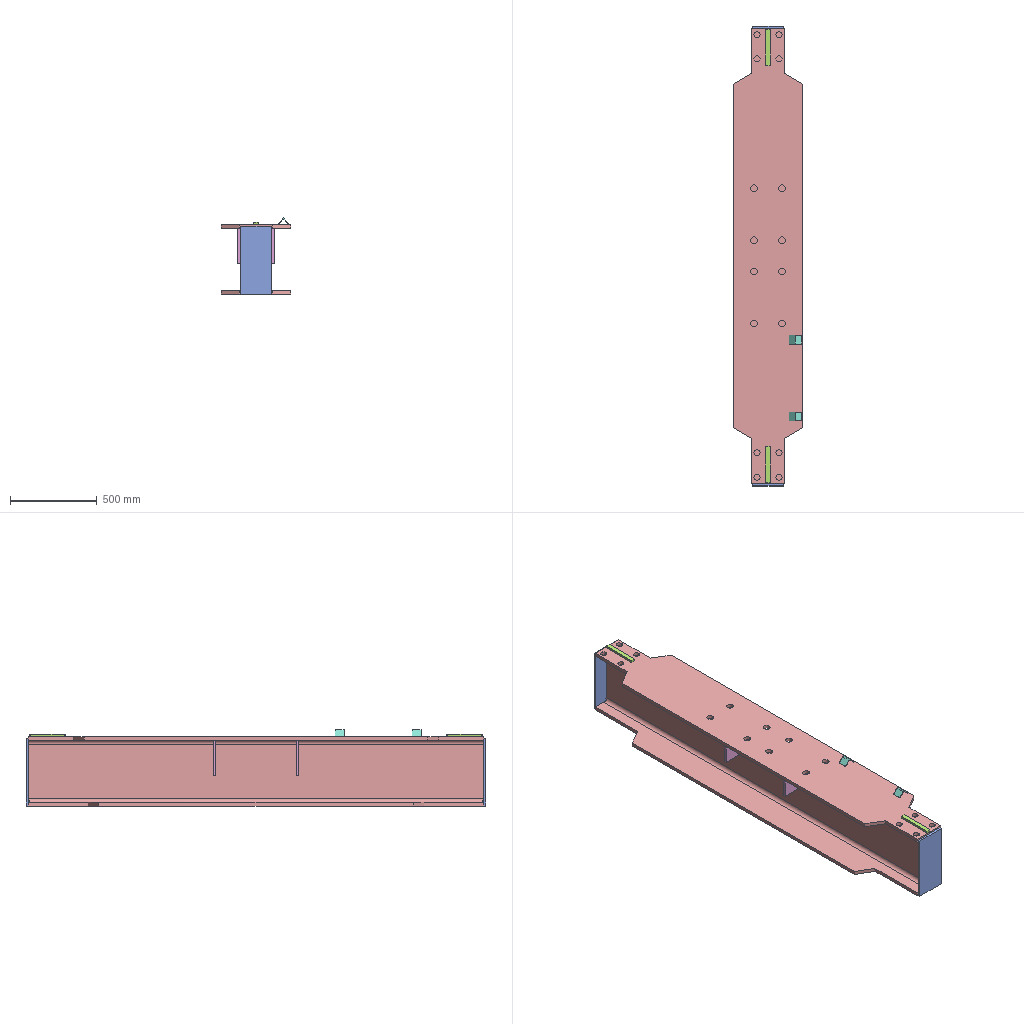Assembly | SolidWorks | 5 different items | 11 placed | box 400 x 2649 x 438 mm
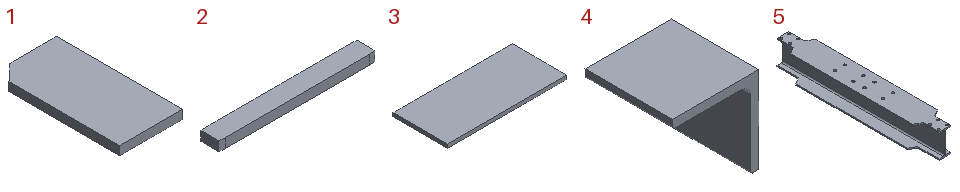Parts list (item | quantity | size | volume | features):
1 | x4 | 101.6 x 203.2 x 14 mm | 284657 mm3 | features Chamfer 1, Extrusion 1
2 | x2 | 209.55 x 25 x 12.7 mm | 66431 mm3 | features Cut 1, Extrusion 1
3 | x2 | 390 x 177.8 x 12 mm | 832104 mm3 | features Extrusion 1
4 | x2 | 50 x 50.8 x 50 mm | 24399 mm3 | features Fillet 2, Extrusion 1
5 | x1 | 400 x 2625 x 400 mm | 51162611 mm3 | features Cut 4, Extrusion 1
Mates (type | each side: item.copy, entity, surface, feature):
Coincident | 3.1 plane | assembly plane
Coincident | 5.1 face plane Extrude1 | 3.1 face plane Extrude1 | 2 times
Coincident | 5.1 face plane Extrude1 | 3.2 face plane Extrude1 | 2 times
Coincident | 3.2 plane | assembly plane
Coincident | 5.1 face plane Extrude1 | 2.1 face plane Extrude1
Coincident | 5.1 face plane Extrude1 | 2.2 face plane Extrude1
Coincident | 2.2 plane | assembly plane
Coincident | 2.1 plane | assembly plane
Symmetric | 2.2 face plane Extrude1 | 2.1 face plane Extrude1 | assembly plane
DistanceDim | 5.1 face plane Extrude1 | 2.2 face plane Extrude1
Coincident | 5.1 face plane Extrude1 | 1.1 face plane Extrude1 | 2 times
Coincident | 5.1 face plane Extrude1 | 1.2 face plane Extrude1 | 2 times
Coincident | 5.1 face plane Extrude1 | 1.3 face plane Extrude1 | 2 times
Coincident | 5.1 face plane Extrude1 | 1.4 face plane Extrude1 | 2 times
Coincident | 1.2 face plane Extrude1 | 1.3 face plane Extrude1
Coincident | 1.1 face plane Extrude1 | 1.4 face plane Extrude1
Symmetric | 1.1 face plane Extrude1 | 1.2 face plane Extrude1 | assembly plane
DistanceDim | 1.1 face plane Extrude1 | 1.2 face plane Extrude1
Tangent | 5.1 face plane Extrude1 | 4.1 face cylinder Fillet2 | 2 times
DistanceDim | 5.1 face plane Extrude1 | 4.1 edge
Coincident | 4.1 face plane Extrude1 | 4.2 face plane Extrude1 | 2 times
DistanceDim | 5.1 face plane Extrude1 | 4.1 face plane Extrude1
DistanceDim | 4.2 face plane Extrude1 | assembly plane